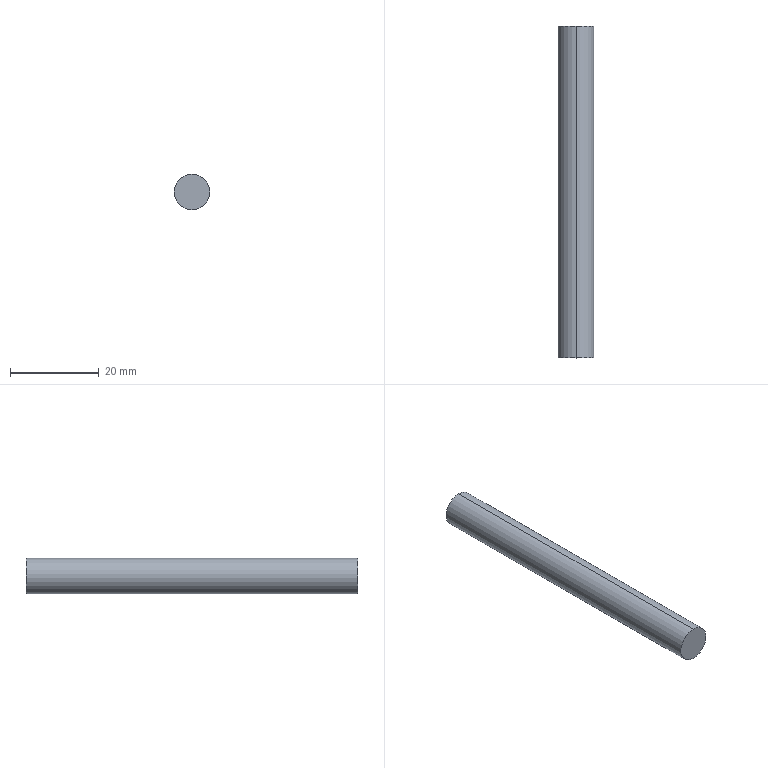Part | SolidWorks | features Extrusion 1, HoleWzd 1 | 1 solid | 8 faces | box 8 x 75 x 8 mm | volume 3681 mm3 | cylinder 4 | cone 2 | plane 2 | commonest cylinder face diameters 3.3 x2 8 x2
STEP:
#1=CARTESIAN_POINT('',(0.,64.9,-1.65));
#2=VERTEX_POINT('',#1);
#3=CARTESIAN_POINT('',(0.,64.9,1.65));
#4=VERTEX_POINT('',#3);
#5=CARTESIAN_POINT('',(0.,64.9,0.));
#6=DIRECTION('',(0.,1.,0.));
#7=DIRECTION('',(0.,0.,1.));
#8=AXIS2_PLACEMENT_3D('',#5,#6,#7);
#9=CIRCLE('',#8,1.65);
#10=EDGE_CURVE('',#2,#4,#9,.T.);
#11=ORIENTED_EDGE('',*,*,#10,.F.);
#12=CARTESIAN_POINT('',(0.,75.,-1.65));
#13=VERTEX_POINT('',#12);
#14=CARTESIAN_POINT('',(0.,75.,-1.65));
#15=DIRECTION('',(0.,1.,0.));
#16=VECTOR('',#15,1000.);
#17=LINE('',#14,#16);
#18=EDGE_CURVE('',#2,#13,#17,.T.);
#19=ORIENTED_EDGE('',*,*,#18,.T.);
#20=CARTESIAN_POINT('',(0.,75.,1.65));
#21=VERTEX_POINT('',#20);
#22=CARTESIAN_POINT('',(0.,75.,0.));
#23=DIRECTION('',(0.,1.,0.));
#24=DIRECTION('',(0.,0.,1.));
#25=AXIS2_PLACEMENT_3D('',#22,#23,#24);
#26=CIRCLE('',#25,1.65);
#27=EDGE_CURVE('',#13,#21,#26,.T.);
#28=ORIENTED_EDGE('',*,*,#27,.T.);
#29=CARTESIAN_POINT('',(0.,75.,1.65));
#30=DIRECTION('',(0.,1.,0.));
#31=VECTOR('',#30,1000.);
#32=LINE('',#29,#31);
#33=EDGE_CURVE('',#4,#21,#32,.T.);
#34=ORIENTED_EDGE('',*,*,#33,.F.);
#35=EDGE_LOOP('',(#11,#19,#28,#34));
#36=FACE_OUTER_BOUND('',#35,.T.);
#37=CARTESIAN_POINT('',(0.,75.,0.));
#38=DIRECTION('',(0.,1.,0.));
#39=DIRECTION('',(0.,0.,1.));
#40=AXIS2_PLACEMENT_3D('',#37,#38,#39);
#41=CYLINDRICAL_SURFACE('',#40,1.65);
#42=ADVANCED_FACE('',(#36),#41,.F.);
#43=CARTESIAN_POINT('',(0.,63.909,0.));
#44=VERTEX_POINT('',#43);
#45=CARTESIAN_POINT('',(0.,64.9,1.65));
#46=DIRECTION('',(0.,0.515,0.8572));
#47=VECTOR('',#46,1000.);
#48=LINE('',#45,#47);
#49=EDGE_CURVE('',#44,#4,#48,.T.);
#50=ORIENTED_EDGE('',*,*,#49,.F.);
#51=CARTESIAN_POINT('',(0.,64.9,-1.65));
#52=DIRECTION('',(0.,0.515,-0.8572));
#53=VECTOR('',#52,1000.);
#54=LINE('',#51,#53);
#55=EDGE_CURVE('',#44,#2,#54,.T.);
#56=ORIENTED_EDGE('',*,*,#55,.T.);
#57=ORIENTED_EDGE('',*,*,#10,.T.);
#58=EDGE_LOOP('',(#50,#56,#57));
#59=FACE_OUTER_BOUND('',#58,.T.);
#60=CARTESIAN_POINT('',(0.,64.9,0.));
#61=DIRECTION('',(0.,1.,0.));
#62=DIRECTION('',(0.,0.,1.));
#63=AXIS2_PLACEMENT_3D('',#60,#61,#62);
#64=CONICAL_SURFACE('',#63,1.65,1.03);
#65=ADVANCED_FACE('',(#59),#64,.F.);
#66=CARTESIAN_POINT('',(0.,75.,4.));
#67=VERTEX_POINT('',#66);
#68=CARTESIAN_POINT('',(0.,75.,-4.));
#69=VERTEX_POINT('',#68);
#70=CARTESIAN_POINT('',(0.,75.,0.));
#71=DIRECTION('',(0.,1.,0.));
#72=DIRECTION('',(0.,0.,1.));
#73=AXIS2_PLACEMENT_3D('',#70,#71,#72);
#74=CIRCLE('',#73,4.);
#75=EDGE_CURVE('',#67,#69,#74,.T.);
#76=ORIENTED_EDGE('',*,*,#75,.F.);
#77=CARTESIAN_POINT('',(0.,0.,4.));
#78=VERTEX_POINT('',#77);
#79=CARTESIAN_POINT('',(0.,75.,4.));
#80=DIRECTION('',(0.,-1.,0.));
#81=VECTOR('',#80,1000.);
#82=LINE('',#79,#81);
#83=EDGE_CURVE('',#67,#78,#82,.T.);
#84=ORIENTED_EDGE('',*,*,#83,.T.);
#85=CARTESIAN_POINT('',(0.,0.,-4.));
#86=VERTEX_POINT('',#85);
#87=CARTESIAN_POINT('',(0.,0.,0.));
#88=DIRECTION('',(0.,1.,0.));
#89=DIRECTION('',(0.,0.,1.));
#90=AXIS2_PLACEMENT_3D('',#87,#88,#89);
#91=CIRCLE('',#90,4.);
#92=EDGE_CURVE('',#78,#86,#91,.T.);
#93=ORIENTED_EDGE('',*,*,#92,.T.);
#94=CARTESIAN_POINT('',(0.,75.,-4.));
#95=DIRECTION('',(0.,-1.,0.));
#96=VECTOR('',#95,1000.);
#97=LINE('',#94,#96);
#98=EDGE_CURVE('',#69,#86,#97,.T.);
#99=ORIENTED_EDGE('',*,*,#98,.F.);
#100=EDGE_LOOP('',(#76,#84,#93,#99));
#101=FACE_OUTER_BOUND('',#100,.T.);
#102=CARTESIAN_POINT('',(0.,75.,0.));
#103=DIRECTION('',(0.,-1.,0.));
#104=DIRECTION('',(0.,0.,-1.));
#105=AXIS2_PLACEMENT_3D('',#102,#103,#104);
#106=CYLINDRICAL_SURFACE('',#105,4.);
#107=ADVANCED_FACE('',(#101),#106,.T.);
#108=ORIENTED_EDGE('',*,*,#83,.F.);
#109=CARTESIAN_POINT('',(0.,75.,0.));
#110=DIRECTION('',(0.,1.,0.));
#111=DIRECTION('',(0.,0.,1.));
#112=AXIS2_PLACEMENT_3D('',#109,#110,#111);
#113=CIRCLE('',#112,4.);
#114=EDGE_CURVE('',#69,#67,#113,.T.);
#115=ORIENTED_EDGE('',*,*,#114,.F.);
#116=ORIENTED_EDGE('',*,*,#98,.T.);
#117=CARTESIAN_POINT('',(0.,0.,0.));
#118=DIRECTION('',(0.,1.,0.));
#119=DIRECTION('',(0.,0.,1.));
#120=AXIS2_PLACEMENT_3D('',#117,#118,#119);
#121=CIRCLE('',#120,4.);
#122=EDGE_CURVE('',#86,#78,#121,.T.);
#123=ORIENTED_EDGE('',*,*,#122,.T.);
#124=EDGE_LOOP('',(#108,#115,#116,#123));
#125=FACE_OUTER_BOUND('',#124,.T.);
#126=CARTESIAN_POINT('',(0.,75.,0.));
#127=DIRECTION('',(0.,-1.,0.));
#128=DIRECTION('',(0.,0.,-1.));
#129=AXIS2_PLACEMENT_3D('',#126,#127,#128);
#130=CYLINDRICAL_SURFACE('',#129,4.);
#131=ADVANCED_FACE('',(#125),#130,.T.);
#132=CARTESIAN_POINT('',(0.,75.,0.));
#133=DIRECTION('',(0.,1.,0.));
#134=DIRECTION('',(0.,0.,1.));
#135=AXIS2_PLACEMENT_3D('',#132,#133,#134);
#136=CIRCLE('',#135,1.65);
#137=EDGE_CURVE('',#21,#13,#136,.T.);
#138=ORIENTED_EDGE('',*,*,#137,.F.);
#139=ORIENTED_EDGE('',*,*,#27,.F.);
#140=EDGE_LOOP('',(#138,#139));
#141=FACE_BOUND('',#140,.T.);
#142=ORIENTED_EDGE('',*,*,#114,.T.);
#143=ORIENTED_EDGE('',*,*,#75,.T.);
#144=EDGE_LOOP('',(#142,#143));
#145=FACE_OUTER_BOUND('',#144,.T.);
#146=CARTESIAN_POINT('',(0.,75.,0.));
#147=DIRECTION('',(0.,1.,0.));
#148=DIRECTION('',(0.,0.,1.));
#149=AXIS2_PLACEMENT_3D('',#146,#147,#148);
#150=PLANE('',#149);
#151=ADVANCED_FACE('',(#141,#145),#150,.T.);
#152=ORIENTED_EDGE('',*,*,#122,.F.);
#153=ORIENTED_EDGE('',*,*,#92,.F.);
#154=EDGE_LOOP('',(#152,#153));
#155=FACE_OUTER_BOUND('',#154,.T.);
#156=CARTESIAN_POINT('',(0.,0.,0.));
#157=DIRECTION('',(0.,1.,0.));
#158=DIRECTION('',(0.,0.,1.));
#159=AXIS2_PLACEMENT_3D('',#156,#157,#158);
#160=PLANE('',#159);
#161=ADVANCED_FACE('',(#155),#160,.F.);
#162=ORIENTED_EDGE('',*,*,#55,.F.);
#163=ORIENTED_EDGE('',*,*,#49,.T.);
#164=CARTESIAN_POINT('',(0.,64.9,0.));
#165=DIRECTION('',(0.,1.,0.));
#166=DIRECTION('',(0.,0.,1.));
#167=AXIS2_PLACEMENT_3D('',#164,#165,#166);
#168=CIRCLE('',#167,1.65);
#169=EDGE_CURVE('',#4,#2,#168,.T.);
#170=ORIENTED_EDGE('',*,*,#169,.T.);
#171=EDGE_LOOP('',(#162,#163,#170));
#172=FACE_OUTER_BOUND('',#171,.T.);
#173=CARTESIAN_POINT('',(0.,64.9,0.));
#174=DIRECTION('',(0.,1.,0.));
#175=DIRECTION('',(0.,0.,1.));
#176=AXIS2_PLACEMENT_3D('',#173,#174,#175);
#177=CONICAL_SURFACE('',#176,1.65,1.03);
#178=ADVANCED_FACE('',(#172),#177,.F.);
#179=ORIENTED_EDGE('',*,*,#18,.F.);
#180=ORIENTED_EDGE('',*,*,#169,.F.);
#181=ORIENTED_EDGE('',*,*,#33,.T.);
#182=ORIENTED_EDGE('',*,*,#137,.T.);
#183=EDGE_LOOP('',(#179,#180,#181,#182));
#184=FACE_OUTER_BOUND('',#183,.T.);
#185=CARTESIAN_POINT('',(0.,75.,0.));
#186=DIRECTION('',(0.,1.,0.));
#187=DIRECTION('',(0.,0.,1.));
#188=AXIS2_PLACEMENT_3D('',#185,#186,#187);
#189=CYLINDRICAL_SURFACE('',#188,1.65);
#190=ADVANCED_FACE('',(#184),#189,.F.);
#191=CLOSED_SHELL('',(#42,#65,#107,#131,#151,#161,#178,#190));
#192=MANIFOLD_SOLID_BREP('',#191);
#193=CARTESIAN_POINT('',(0.,0.,0.));
#194=DIRECTION('',(0.,0.,1.));
#195=DIRECTION('',(1.,0.,0.));
#196=AXIS2_PLACEMENT_3D('',#193,#194,#195);
#197=(LENGTH_UNIT()NAMED_UNIT(*)SI_UNIT(.MILLI.,.METRE.));
#198=UNCERTAINTY_MEASURE_WITH_UNIT(LENGTH_MEASURE(0.00001),#197,'','');
#199=(NAMED_UNIT(*)PLANE_ANGLE_UNIT()SI_UNIT($,.RADIAN.));
#200=(NAMED_UNIT(*)SI_UNIT($,.STERADIAN.)SOLID_ANGLE_UNIT());
#201=(GEOMETRIC_REPRESENTATION_CONTEXT(3)GLOBAL_UNCERTAINTY_ASSIGNED_CONTEXT((#198))GLOBAL_UNIT_ASSIGNED_CONTEXT((#197,#199,#200))REPRESENTATION_CONTEXT('',''));
#202=ADVANCED_BREP_SHAPE_REPRESENTATION('',(#192,#196),#201);